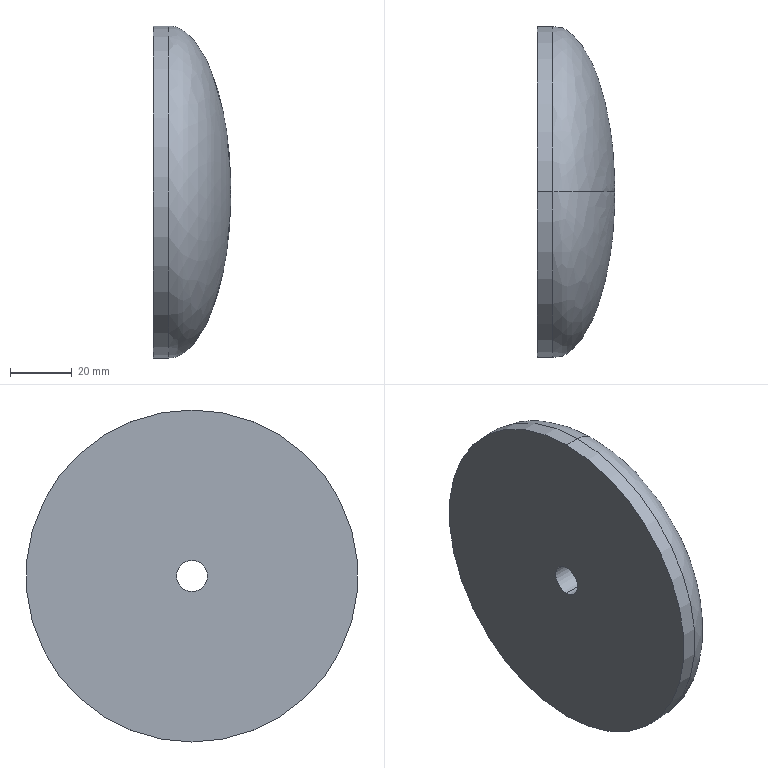Part | SolidWorks | features BaseBody 1 | 1 solid | 7 faces | box 24.913 x 107.2 x 107.2 mm | volume 163511 mm3 | cylinder 4 | spline 2 | plane 1 | commonest cylinder face diameters 10 x2 107.2 x2
STEP:
#1=CARTESIAN_POINT('',(24.913,0.,5.));
#2=VERTEX_POINT('',#1);
#3=CARTESIAN_POINT('',(24.913,0.,-5.));
#4=VERTEX_POINT('',#3);
#5=CARTESIAN_POINT('',(24.913,0.,0.));
#6=DIRECTION('',(1.,0.,0.));
#7=DIRECTION('',(0.,0.,-1.));
#8=AXIS2_PLACEMENT_3D('',#5,#6,#7);
#9=CIRCLE('',#8,5.);
#10=EDGE_CURVE('',#2,#4,#9,.T.);
#11=ORIENTED_EDGE('',*,*,#10,.F.);
#12=CARTESIAN_POINT('',(5.,0.,53.6));
#13=VERTEX_POINT('',#12);
#14=CARTESIAN_POINT('',(24.913,0.,5.));
#15=CARTESIAN_POINT('',(23.899,0.,33.993));
#16=CARTESIAN_POINT('',(15.866,0.,53.6));
#17=CARTESIAN_POINT('',(5.,0.,53.6));
#18=(BOUNDED_CURVE()B_SPLINE_CURVE(3,(#14,#15,#16,#17),.UNSPECIFIED.,.F.,.T.)B_SPLINE_CURVE_WITH_KNOTS((4,4),(4.806,6.283),.UNSPECIFIED.)CURVE()GEOMETRIC_REPRESENTATION_ITEM()RATIONAL_B_SPLINE_CURVE((1.,0.8262,0.8262,1.))REPRESENTATION_ITEM(''));
#19=EDGE_CURVE('',#2,#13,#18,.T.);
#20=ORIENTED_EDGE('',*,*,#19,.T.);
#21=CARTESIAN_POINT('',(5.,0.,-53.6));
#22=VERTEX_POINT('',#21);
#23=CARTESIAN_POINT('',(5.,0.,0.));
#24=DIRECTION('',(1.,0.,0.));
#25=DIRECTION('',(0.,0.,-1.));
#26=AXIS2_PLACEMENT_3D('',#23,#24,#25);
#27=CIRCLE('',#26,53.6);
#28=EDGE_CURVE('',#13,#22,#27,.T.);
#29=ORIENTED_EDGE('',*,*,#28,.T.);
#30=CARTESIAN_POINT('',(24.913,0.,-5.));
#31=CARTESIAN_POINT('',(23.899,0.,-33.993));
#32=CARTESIAN_POINT('',(15.866,0.,-53.6));
#33=CARTESIAN_POINT('',(5.,0.,-53.6));
#34=(BOUNDED_CURVE()B_SPLINE_CURVE(3,(#30,#31,#32,#33),.UNSPECIFIED.,.F.,.F.)B_SPLINE_CURVE_WITH_KNOTS((4,4),(4.806,6.283),.UNSPECIFIED.)CURVE()GEOMETRIC_REPRESENTATION_ITEM()RATIONAL_B_SPLINE_CURVE((1.,0.8262,0.8262,1.))REPRESENTATION_ITEM(''));
#35=EDGE_CURVE('',#4,#22,#34,.T.);
#36=ORIENTED_EDGE('',*,*,#35,.F.);
#37=EDGE_LOOP('',(#11,#20,#29,#36));
#38=FACE_OUTER_BOUND('',#37,.T.);
#39=CARTESIAN_POINT('',(24.913,0.,5.));
#40=CARTESIAN_POINT('',(24.913,-10.,5.));
#41=CARTESIAN_POINT('',(24.913,-10.,-5.));
#42=CARTESIAN_POINT('',(24.913,0.,-5.));
#43=CARTESIAN_POINT('',(23.899,0.,33.993));
#44=CARTESIAN_POINT('',(23.899,-67.986,33.993));
#45=CARTESIAN_POINT('',(23.899,-67.986,-33.993));
#46=CARTESIAN_POINT('',(23.899,0.,-33.993));
#47=CARTESIAN_POINT('',(15.866,0.,53.6));
#48=CARTESIAN_POINT('',(15.866,-107.2,53.6));
#49=CARTESIAN_POINT('',(15.866,-107.2,-53.6));
#50=CARTESIAN_POINT('',(15.866,0.,-53.6));
#51=CARTESIAN_POINT('',(5.,0.,53.6));
#52=CARTESIAN_POINT('',(5.,-107.2,53.6));
#53=CARTESIAN_POINT('',(5.,-107.2,-53.6));
#54=CARTESIAN_POINT('',(5.,0.,-53.6));
#55=(BOUNDED_SURFACE()B_SPLINE_SURFACE(3,3,((#39,#40,#41,#42),(#43,#44,#45,#46),(#47,#48,#49,#50),(#51,#52,#53,#54)),.UNSPECIFIED.,.F.,.F.,.T.)B_SPLINE_SURFACE_WITH_KNOTS((4,4),(4,4),(0.,1.),(0.,1.),.UNSPECIFIED.)GEOMETRIC_REPRESENTATION_ITEM()RATIONAL_B_SPLINE_SURFACE(((1.,0.3333,0.3333,1.),(0.8262,0.2754,0.2754,0.8262),(0.8262,0.2754,0.2754,0.8262),(1.,0.3333,0.3333,1.)))REPRESENTATION_ITEM('')SURFACE());
#56=ADVANCED_FACE('',(#38),#55,.T.);
#57=ORIENTED_EDGE('',*,*,#10,.T.);
#58=CARTESIAN_POINT('',(0.,0.,-5.));
#59=VERTEX_POINT('',#58);
#60=CARTESIAN_POINT('',(25.,0.,-5.));
#61=DIRECTION('',(-1.,0.,0.));
#62=VECTOR('',#61,1000.);
#63=LINE('',#60,#62);
#64=EDGE_CURVE('',#4,#59,#63,.T.);
#65=ORIENTED_EDGE('',*,*,#64,.T.);
#66=CARTESIAN_POINT('',(0.,0.,5.));
#67=VERTEX_POINT('',#66);
#68=CARTESIAN_POINT('',(0.,0.,0.));
#69=DIRECTION('',(-1.,0.,0.));
#70=DIRECTION('',(0.,0.,1.));
#71=AXIS2_PLACEMENT_3D('',#68,#69,#70);
#72=CIRCLE('',#71,5.);
#73=EDGE_CURVE('',#59,#67,#72,.T.);
#74=ORIENTED_EDGE('',*,*,#73,.T.);
#75=CARTESIAN_POINT('',(25.,0.,5.));
#76=DIRECTION('',(-1.,0.,0.));
#77=VECTOR('',#76,1000.);
#78=LINE('',#75,#77);
#79=EDGE_CURVE('',#2,#67,#78,.T.);
#80=ORIENTED_EDGE('',*,*,#79,.F.);
#81=EDGE_LOOP('',(#57,#65,#74,#80));
#82=FACE_OUTER_BOUND('',#81,.T.);
#83=CARTESIAN_POINT('',(25.,0.,0.));
#84=DIRECTION('',(-1.,0.,0.));
#85=DIRECTION('',(0.,0.,1.));
#86=AXIS2_PLACEMENT_3D('',#83,#84,#85);
#87=CYLINDRICAL_SURFACE('',#86,5.);
#88=ADVANCED_FACE('',(#82),#87,.F.);
#89=CARTESIAN_POINT('',(5.,0.,0.));
#90=DIRECTION('',(1.,0.,0.));
#91=DIRECTION('',(0.,0.,-1.));
#92=AXIS2_PLACEMENT_3D('',#89,#90,#91);
#93=CIRCLE('',#92,53.6);
#94=EDGE_CURVE('',#22,#13,#93,.T.);
#95=ORIENTED_EDGE('',*,*,#94,.F.);
#96=CARTESIAN_POINT('',(0.,0.,-53.6));
#97=VERTEX_POINT('',#96);
#98=CARTESIAN_POINT('',(5.,0.,-53.6));
#99=DIRECTION('',(-1.,0.,0.));
#100=VECTOR('',#99,1000.);
#101=LINE('',#98,#100);
#102=EDGE_CURVE('',#22,#97,#101,.T.);
#103=ORIENTED_EDGE('',*,*,#102,.T.);
#104=CARTESIAN_POINT('',(0.,0.,53.6));
#105=VERTEX_POINT('',#104);
#106=CARTESIAN_POINT('',(0.,0.,0.));
#107=DIRECTION('',(1.,0.,0.));
#108=DIRECTION('',(0.,0.,-1.));
#109=AXIS2_PLACEMENT_3D('',#106,#107,#108);
#110=CIRCLE('',#109,53.6);
#111=EDGE_CURVE('',#97,#105,#110,.T.);
#112=ORIENTED_EDGE('',*,*,#111,.T.);
#113=CARTESIAN_POINT('',(5.,0.,53.6));
#114=DIRECTION('',(-1.,0.,0.));
#115=VECTOR('',#114,1000.);
#116=LINE('',#113,#115);
#117=EDGE_CURVE('',#13,#105,#116,.T.);
#118=ORIENTED_EDGE('',*,*,#117,.F.);
#119=EDGE_LOOP('',(#95,#103,#112,#118));
#120=FACE_OUTER_BOUND('',#119,.T.);
#121=CARTESIAN_POINT('',(5.,0.,0.));
#122=DIRECTION('',(-1.,0.,0.));
#123=DIRECTION('',(0.,0.,1.));
#124=AXIS2_PLACEMENT_3D('',#121,#122,#123);
#125=CYLINDRICAL_SURFACE('',#124,53.6);
#126=ADVANCED_FACE('',(#120),#125,.T.);
#127=ORIENTED_EDGE('',*,*,#102,.F.);
#128=ORIENTED_EDGE('',*,*,#28,.F.);
#129=ORIENTED_EDGE('',*,*,#117,.T.);
#130=CARTESIAN_POINT('',(0.,0.,0.));
#131=DIRECTION('',(1.,0.,0.));
#132=DIRECTION('',(0.,0.,-1.));
#133=AXIS2_PLACEMENT_3D('',#130,#131,#132);
#134=CIRCLE('',#133,53.6);
#135=EDGE_CURVE('',#105,#97,#134,.T.);
#136=ORIENTED_EDGE('',*,*,#135,.T.);
#137=EDGE_LOOP('',(#127,#128,#129,#136));
#138=FACE_OUTER_BOUND('',#137,.T.);
#139=CARTESIAN_POINT('',(5.,0.,0.));
#140=DIRECTION('',(-1.,0.,0.));
#141=DIRECTION('',(0.,0.,1.));
#142=AXIS2_PLACEMENT_3D('',#139,#140,#141);
#143=CYLINDRICAL_SURFACE('',#142,53.6);
#144=ADVANCED_FACE('',(#138),#143,.T.);
#145=ORIENTED_EDGE('',*,*,#19,.F.);
#146=CARTESIAN_POINT('',(24.913,0.,0.));
#147=DIRECTION('',(1.,0.,0.));
#148=DIRECTION('',(0.,0.,-1.));
#149=AXIS2_PLACEMENT_3D('',#146,#147,#148);
#150=CIRCLE('',#149,5.);
#151=EDGE_CURVE('',#4,#2,#150,.T.);
#152=ORIENTED_EDGE('',*,*,#151,.F.);
#153=ORIENTED_EDGE('',*,*,#35,.T.);
#154=ORIENTED_EDGE('',*,*,#94,.T.);
#155=EDGE_LOOP('',(#145,#152,#153,#154));
#156=FACE_OUTER_BOUND('',#155,.T.);
#157=CARTESIAN_POINT('',(24.913,0.,-5.));
#158=CARTESIAN_POINT('',(24.913,10.,-5.));
#159=CARTESIAN_POINT('',(24.913,10.,5.));
#160=CARTESIAN_POINT('',(24.913,0.,5.));
#161=CARTESIAN_POINT('',(23.899,0.,-33.993));
#162=CARTESIAN_POINT('',(23.899,67.986,-33.993));
#163=CARTESIAN_POINT('',(23.899,67.986,33.993));
#164=CARTESIAN_POINT('',(23.899,0.,33.993));
#165=CARTESIAN_POINT('',(15.866,0.,-53.6));
#166=CARTESIAN_POINT('',(15.866,107.2,-53.6));
#167=CARTESIAN_POINT('',(15.866,107.2,53.6));
#168=CARTESIAN_POINT('',(15.866,0.,53.6));
#169=CARTESIAN_POINT('',(5.,0.,-53.6));
#170=CARTESIAN_POINT('',(5.,107.2,-53.6));
#171=CARTESIAN_POINT('',(5.,107.2,53.6));
#172=CARTESIAN_POINT('',(5.,0.,53.6));
#173=(BOUNDED_SURFACE()B_SPLINE_SURFACE(3,3,((#157,#158,#159,#160),(#161,#162,#163,#164),(#165,#166,#167,#168),(#169,#170,#171,#172)),.UNSPECIFIED.,.F.,.F.,.F.)B_SPLINE_SURFACE_WITH_KNOTS((4,4),(4,4),(0.,1.),(0.,1.),.UNSPECIFIED.)GEOMETRIC_REPRESENTATION_ITEM()RATIONAL_B_SPLINE_SURFACE(((1.,0.3333,0.3333,1.),(0.8262,0.2754,0.2754,0.8262),(0.8262,0.2754,0.2754,0.8262),(1.,0.3333,0.3333,1.)))REPRESENTATION_ITEM('')SURFACE());
#174=ADVANCED_FACE('',(#156),#173,.T.);
#175=ORIENTED_EDGE('',*,*,#135,.F.);
#176=ORIENTED_EDGE('',*,*,#111,.F.);
#177=EDGE_LOOP('',(#175,#176));
#178=FACE_OUTER_BOUND('',#177,.T.);
#179=CARTESIAN_POINT('',(0.,0.,0.));
#180=DIRECTION('',(-1.,0.,0.));
#181=DIRECTION('',(0.,0.,1.));
#182=AXIS2_PLACEMENT_3D('',#179,#180,#181);
#183=CIRCLE('',#182,5.);
#184=EDGE_CURVE('',#67,#59,#183,.T.);
#185=ORIENTED_EDGE('',*,*,#184,.F.);
#186=ORIENTED_EDGE('',*,*,#73,.F.);
#187=EDGE_LOOP('',(#185,#186));
#188=FACE_BOUND('',#187,.T.);
#189=CARTESIAN_POINT('',(0.,0.,0.));
#190=DIRECTION('',(1.,0.,0.));
#191=DIRECTION('',(0.,1.,0.));
#192=AXIS2_PLACEMENT_3D('',#189,#190,#191);
#193=PLANE('',#192);
#194=ADVANCED_FACE('',(#178,#188),#193,.F.);
#195=ORIENTED_EDGE('',*,*,#64,.F.);
#196=ORIENTED_EDGE('',*,*,#151,.T.);
#197=ORIENTED_EDGE('',*,*,#79,.T.);
#198=ORIENTED_EDGE('',*,*,#184,.T.);
#199=EDGE_LOOP('',(#195,#196,#197,#198));
#200=FACE_OUTER_BOUND('',#199,.T.);
#201=CARTESIAN_POINT('',(25.,0.,0.));
#202=DIRECTION('',(-1.,0.,0.));
#203=DIRECTION('',(0.,0.,1.));
#204=AXIS2_PLACEMENT_3D('',#201,#202,#203);
#205=CYLINDRICAL_SURFACE('',#204,5.);
#206=ADVANCED_FACE('',(#200),#205,.F.);
#207=CLOSED_SHELL('',(#56,#88,#126,#144,#174,#194,#206));
#208=MANIFOLD_SOLID_BREP('',#207);
#209=CARTESIAN_POINT('',(0.,0.,0.));
#210=DIRECTION('',(0.,0.,1.));
#211=DIRECTION('',(1.,0.,0.));
#212=AXIS2_PLACEMENT_3D('',#209,#210,#211);
#213=(LENGTH_UNIT()NAMED_UNIT(*)SI_UNIT(.MILLI.,.METRE.));
#214=UNCERTAINTY_MEASURE_WITH_UNIT(LENGTH_MEASURE(0.00001),#213,'','');
#215=(NAMED_UNIT(*)PLANE_ANGLE_UNIT()SI_UNIT($,.RADIAN.));
#216=(NAMED_UNIT(*)SI_UNIT($,.STERADIAN.)SOLID_ANGLE_UNIT());
#217=(GEOMETRIC_REPRESENTATION_CONTEXT(3)GLOBAL_UNCERTAINTY_ASSIGNED_CONTEXT((#214))GLOBAL_UNIT_ASSIGNED_CONTEXT((#213,#215,#216))REPRESENTATION_CONTEXT('',''));
#218=ADVANCED_BREP_SHAPE_REPRESENTATION('',(#208,#212),#217);